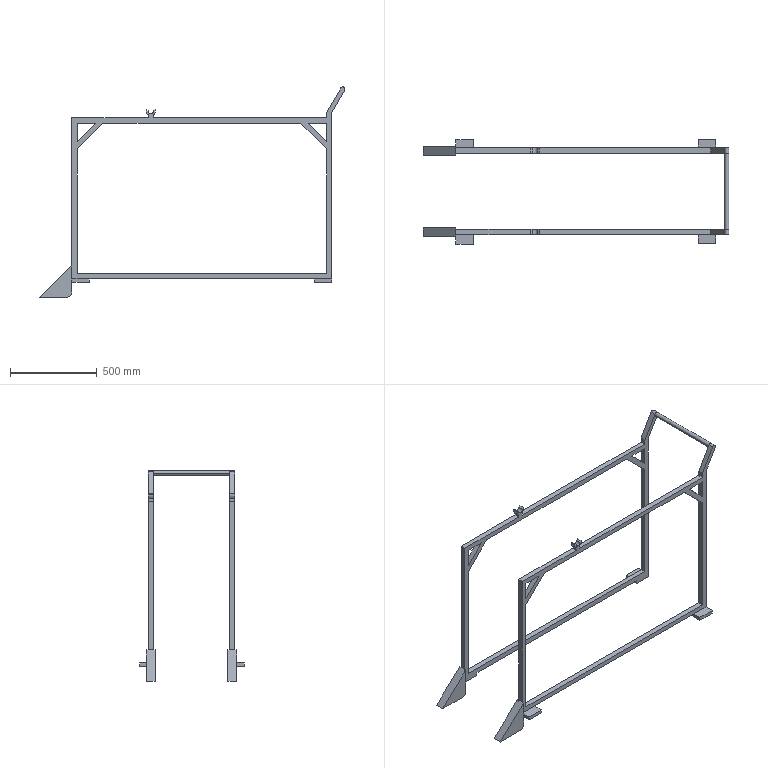Part | SolidWorks | features ICE 12, MirrorPattern 4, Extrusion 1, Fillet 1 | 1 solid | 103 faces | box 1767 x 605.941 x 1214 mm | volume 12147544 mm3 | plane 84 | cylinder 19 | commonest cylinder face diameters 30.122 x6 53.031 x6 25.983 x3 25.981 x2 60 x2